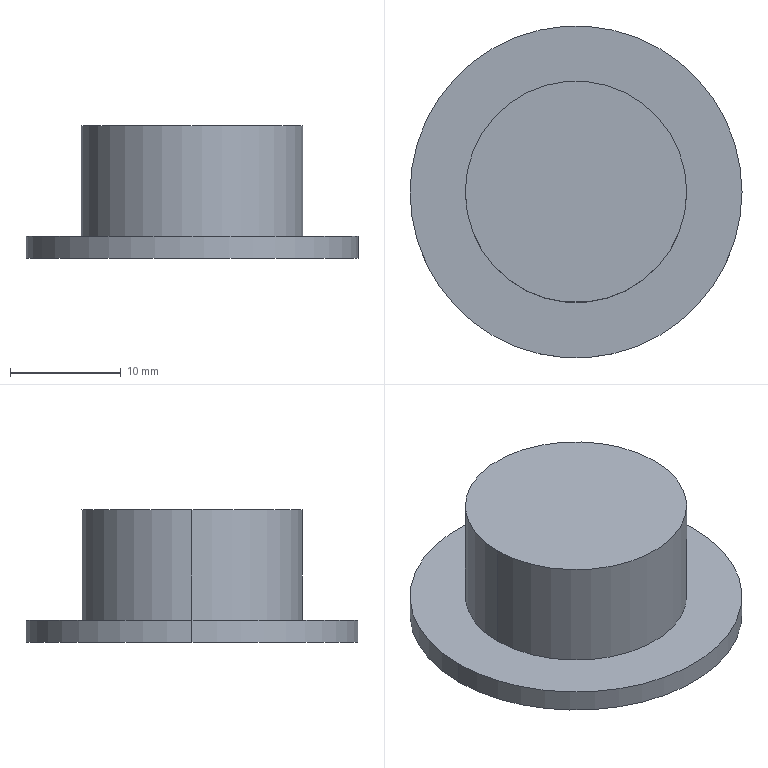Part | SolidWorks | features Extrusion 1, ICE 1 | 1 solid | 7 faces | box 30 x 30 x 12 mm | volume 4555 mm3 | cylinder 4 | plane 3 | commonest cylinder face diameters 20 x2 30 x2
STEP:
#1=CARTESIAN_POINT('',(10.,0.,12.));
#2=VERTEX_POINT('',#1);
#3=CARTESIAN_POINT('',(-10.,0.,12.));
#4=VERTEX_POINT('',#3);
#5=CARTESIAN_POINT('',(0.,0.,12.));
#6=DIRECTION('',(0.,0.,1.));
#7=DIRECTION('',(1.,0.,0.));
#8=AXIS2_PLACEMENT_3D('',#5,#6,#7);
#9=CIRCLE('',#8,10.);
#10=EDGE_CURVE('',#2,#4,#9,.T.);
#11=ORIENTED_EDGE('',*,*,#10,.F.);
#12=CARTESIAN_POINT('',(10.,0.,2.));
#13=VERTEX_POINT('',#12);
#14=CARTESIAN_POINT('',(10.,0.,12.));
#15=DIRECTION('',(0.,0.,-1.));
#16=VECTOR('',#15,1000.);
#17=LINE('',#14,#16);
#18=EDGE_CURVE('',#2,#13,#17,.T.);
#19=ORIENTED_EDGE('',*,*,#18,.T.);
#20=CARTESIAN_POINT('',(-10.,0.,2.));
#21=VERTEX_POINT('',#20);
#22=CARTESIAN_POINT('',(0.,0.,2.));
#23=DIRECTION('',(0.,0.,1.));
#24=DIRECTION('',(1.,0.,0.));
#25=AXIS2_PLACEMENT_3D('',#22,#23,#24);
#26=CIRCLE('',#25,10.);
#27=EDGE_CURVE('',#13,#21,#26,.T.);
#28=ORIENTED_EDGE('',*,*,#27,.T.);
#29=CARTESIAN_POINT('',(-10.,0.,12.));
#30=DIRECTION('',(0.,0.,-1.));
#31=VECTOR('',#30,1000.);
#32=LINE('',#29,#31);
#33=EDGE_CURVE('',#4,#21,#32,.T.);
#34=ORIENTED_EDGE('',*,*,#33,.F.);
#35=EDGE_LOOP('',(#11,#19,#28,#34));
#36=FACE_OUTER_BOUND('',#35,.T.);
#37=CARTESIAN_POINT('',(0.,0.,12.));
#38=DIRECTION('',(0.,0.,-1.));
#39=DIRECTION('',(-1.,0.,0.));
#40=AXIS2_PLACEMENT_3D('',#37,#38,#39);
#41=CYLINDRICAL_SURFACE('',#40,10.);
#42=ADVANCED_FACE('',(#36),#41,.T.);
#43=CARTESIAN_POINT('',(15.,0.,2.));
#44=VERTEX_POINT('',#43);
#45=CARTESIAN_POINT('',(-15.,0.,2.));
#46=VERTEX_POINT('',#45);
#47=CARTESIAN_POINT('',(0.,0.,2.));
#48=DIRECTION('',(0.,0.,1.));
#49=DIRECTION('',(1.,0.,0.));
#50=AXIS2_PLACEMENT_3D('',#47,#48,#49);
#51=CIRCLE('',#50,15.);
#52=EDGE_CURVE('',#44,#46,#51,.T.);
#53=ORIENTED_EDGE('',*,*,#52,.F.);
#54=CARTESIAN_POINT('',(15.,0.,0.));
#55=VERTEX_POINT('',#54);
#56=CARTESIAN_POINT('',(15.,0.,2.));
#57=DIRECTION('',(0.,0.,-1.));
#58=VECTOR('',#57,1000.);
#59=LINE('',#56,#58);
#60=EDGE_CURVE('',#44,#55,#59,.T.);
#61=ORIENTED_EDGE('',*,*,#60,.T.);
#62=CARTESIAN_POINT('',(-15.,0.,0.));
#63=VERTEX_POINT('',#62);
#64=CARTESIAN_POINT('',(0.,0.,0.));
#65=DIRECTION('',(0.,0.,1.));
#66=DIRECTION('',(1.,0.,0.));
#67=AXIS2_PLACEMENT_3D('',#64,#65,#66);
#68=CIRCLE('',#67,15.);
#69=EDGE_CURVE('',#55,#63,#68,.T.);
#70=ORIENTED_EDGE('',*,*,#69,.T.);
#71=CARTESIAN_POINT('',(-15.,0.,2.));
#72=DIRECTION('',(0.,0.,-1.));
#73=VECTOR('',#72,1000.);
#74=LINE('',#71,#73);
#75=EDGE_CURVE('',#46,#63,#74,.T.);
#76=ORIENTED_EDGE('',*,*,#75,.F.);
#77=EDGE_LOOP('',(#53,#61,#70,#76));
#78=FACE_OUTER_BOUND('',#77,.T.);
#79=CARTESIAN_POINT('',(0.,0.,2.));
#80=DIRECTION('',(0.,0.,-1.));
#81=DIRECTION('',(-1.,0.,0.));
#82=AXIS2_PLACEMENT_3D('',#79,#80,#81);
#83=CYLINDRICAL_SURFACE('',#82,15.);
#84=ADVANCED_FACE('',(#78),#83,.T.);
#85=ORIENTED_EDGE('',*,*,#60,.F.);
#86=CARTESIAN_POINT('',(0.,0.,2.));
#87=DIRECTION('',(0.,0.,1.));
#88=DIRECTION('',(1.,0.,0.));
#89=AXIS2_PLACEMENT_3D('',#86,#87,#88);
#90=CIRCLE('',#89,15.);
#91=EDGE_CURVE('',#46,#44,#90,.T.);
#92=ORIENTED_EDGE('',*,*,#91,.F.);
#93=ORIENTED_EDGE('',*,*,#75,.T.);
#94=CARTESIAN_POINT('',(0.,0.,0.));
#95=DIRECTION('',(0.,0.,1.));
#96=DIRECTION('',(1.,0.,0.));
#97=AXIS2_PLACEMENT_3D('',#94,#95,#96);
#98=CIRCLE('',#97,15.);
#99=EDGE_CURVE('',#63,#55,#98,.T.);
#100=ORIENTED_EDGE('',*,*,#99,.T.);
#101=EDGE_LOOP('',(#85,#92,#93,#100));
#102=FACE_OUTER_BOUND('',#101,.T.);
#103=CARTESIAN_POINT('',(0.,0.,2.));
#104=DIRECTION('',(0.,0.,-1.));
#105=DIRECTION('',(-1.,0.,0.));
#106=AXIS2_PLACEMENT_3D('',#103,#104,#105);
#107=CYLINDRICAL_SURFACE('',#106,15.);
#108=ADVANCED_FACE('',(#102),#107,.T.);
#109=CARTESIAN_POINT('',(0.,0.,2.));
#110=DIRECTION('',(0.,0.,1.));
#111=DIRECTION('',(1.,0.,0.));
#112=AXIS2_PLACEMENT_3D('',#109,#110,#111);
#113=CIRCLE('',#112,10.);
#114=EDGE_CURVE('',#21,#13,#113,.T.);
#115=ORIENTED_EDGE('',*,*,#114,.F.);
#116=ORIENTED_EDGE('',*,*,#27,.F.);
#117=EDGE_LOOP('',(#115,#116));
#118=FACE_BOUND('',#117,.T.);
#119=ORIENTED_EDGE('',*,*,#91,.T.);
#120=ORIENTED_EDGE('',*,*,#52,.T.);
#121=EDGE_LOOP('',(#119,#120));
#122=FACE_OUTER_BOUND('',#121,.T.);
#123=CARTESIAN_POINT('',(0.,0.,2.));
#124=DIRECTION('',(0.,0.,1.));
#125=DIRECTION('',(1.,0.,0.));
#126=AXIS2_PLACEMENT_3D('',#123,#124,#125);
#127=PLANE('',#126);
#128=ADVANCED_FACE('',(#118,#122),#127,.T.);
#129=ORIENTED_EDGE('',*,*,#99,.F.);
#130=ORIENTED_EDGE('',*,*,#69,.F.);
#131=EDGE_LOOP('',(#129,#130));
#132=FACE_OUTER_BOUND('',#131,.T.);
#133=CARTESIAN_POINT('',(0.,0.,0.));
#134=DIRECTION('',(0.,0.,1.));
#135=DIRECTION('',(1.,0.,0.));
#136=AXIS2_PLACEMENT_3D('',#133,#134,#135);
#137=PLANE('',#136);
#138=ADVANCED_FACE('',(#132),#137,.F.);
#139=ORIENTED_EDGE('',*,*,#18,.F.);
#140=CARTESIAN_POINT('',(0.,0.,12.));
#141=DIRECTION('',(0.,0.,1.));
#142=DIRECTION('',(1.,0.,0.));
#143=AXIS2_PLACEMENT_3D('',#140,#141,#142);
#144=CIRCLE('',#143,10.);
#145=EDGE_CURVE('',#4,#2,#144,.T.);
#146=ORIENTED_EDGE('',*,*,#145,.F.);
#147=ORIENTED_EDGE('',*,*,#33,.T.);
#148=ORIENTED_EDGE('',*,*,#114,.T.);
#149=EDGE_LOOP('',(#139,#146,#147,#148));
#150=FACE_OUTER_BOUND('',#149,.T.);
#151=CARTESIAN_POINT('',(0.,0.,12.));
#152=DIRECTION('',(0.,0.,-1.));
#153=DIRECTION('',(-1.,0.,0.));
#154=AXIS2_PLACEMENT_3D('',#151,#152,#153);
#155=CYLINDRICAL_SURFACE('',#154,10.);
#156=ADVANCED_FACE('',(#150),#155,.T.);
#157=ORIENTED_EDGE('',*,*,#145,.T.);
#158=ORIENTED_EDGE('',*,*,#10,.T.);
#159=EDGE_LOOP('',(#157,#158));
#160=FACE_OUTER_BOUND('',#159,.T.);
#161=CARTESIAN_POINT('',(0.,0.,12.));
#162=DIRECTION('',(0.,0.,1.));
#163=DIRECTION('',(1.,0.,0.));
#164=AXIS2_PLACEMENT_3D('',#161,#162,#163);
#165=PLANE('',#164);
#166=ADVANCED_FACE('',(#160),#165,.T.);
#167=CLOSED_SHELL('',(#42,#84,#108,#128,#138,#156,#166));
#168=MANIFOLD_SOLID_BREP('',#167);
#169=CARTESIAN_POINT('',(0.,0.,0.));
#170=DIRECTION('',(0.,0.,1.));
#171=DIRECTION('',(1.,0.,0.));
#172=AXIS2_PLACEMENT_3D('',#169,#170,#171);
#173=(LENGTH_UNIT()NAMED_UNIT(*)SI_UNIT(.MILLI.,.METRE.));
#174=UNCERTAINTY_MEASURE_WITH_UNIT(LENGTH_MEASURE(0.00001),#173,'','');
#175=(NAMED_UNIT(*)PLANE_ANGLE_UNIT()SI_UNIT($,.RADIAN.));
#176=(NAMED_UNIT(*)SI_UNIT($,.STERADIAN.)SOLID_ANGLE_UNIT());
#177=(GEOMETRIC_REPRESENTATION_CONTEXT(3)GLOBAL_UNCERTAINTY_ASSIGNED_CONTEXT((#174))GLOBAL_UNIT_ASSIGNED_CONTEXT((#173,#175,#176))REPRESENTATION_CONTEXT('',''));
#178=ADVANCED_BREP_SHAPE_REPRESENTATION('',(#168,#172),#177);